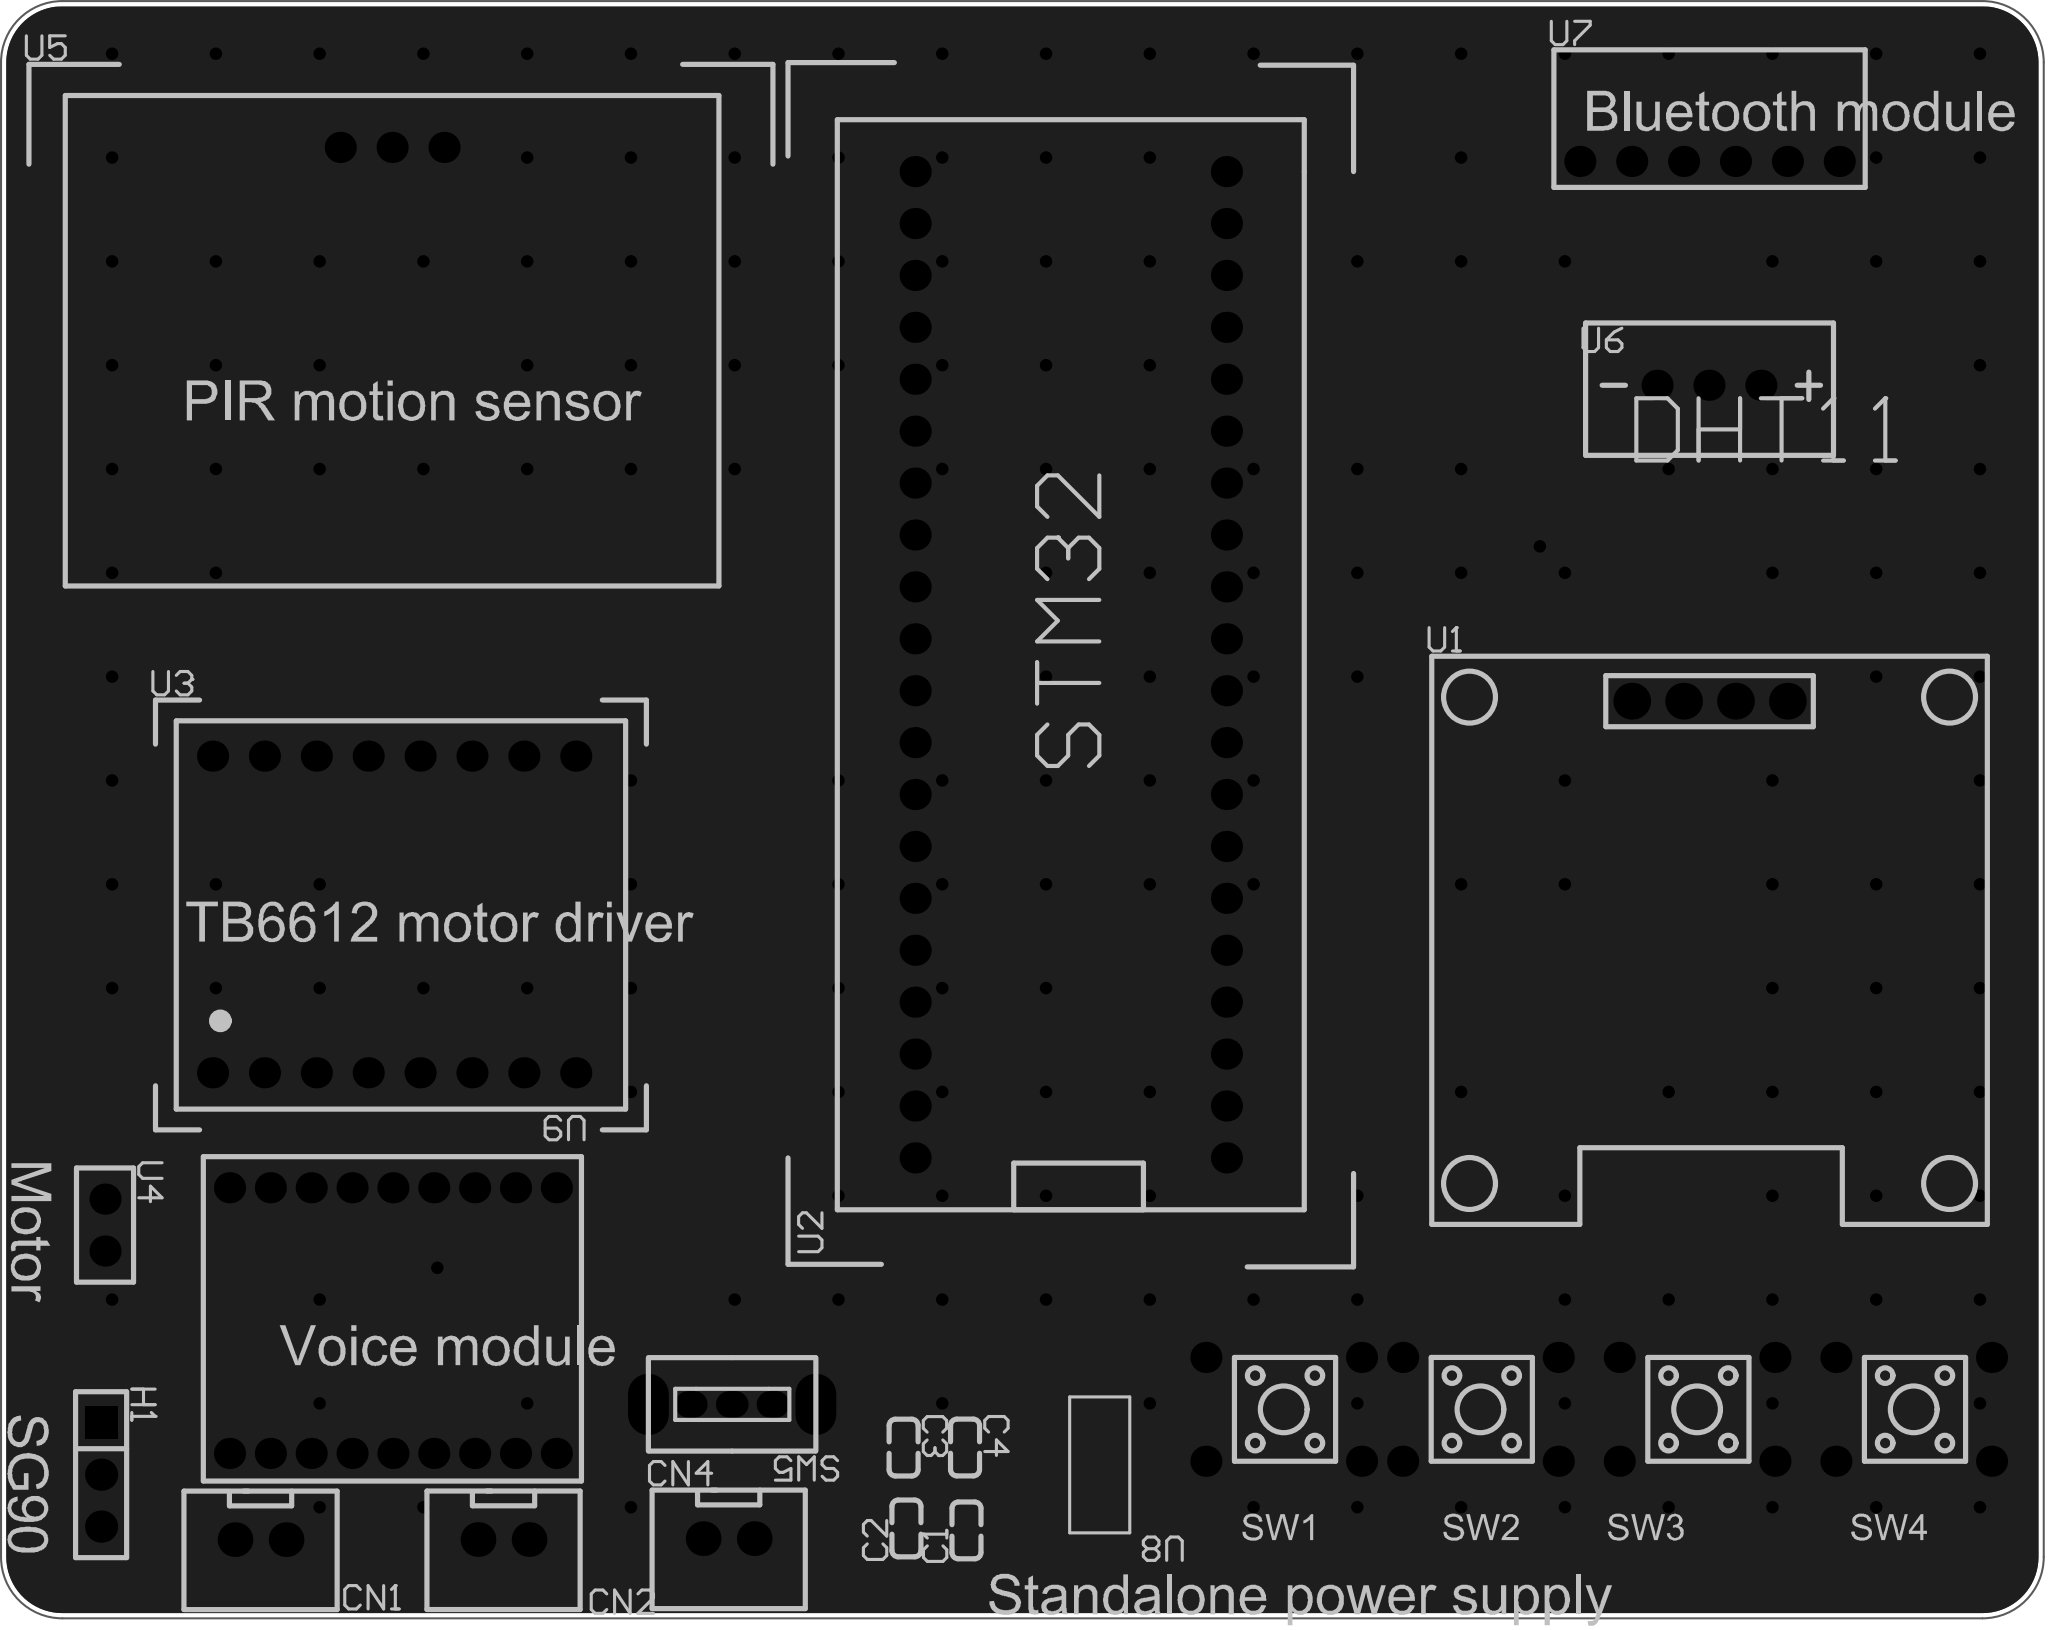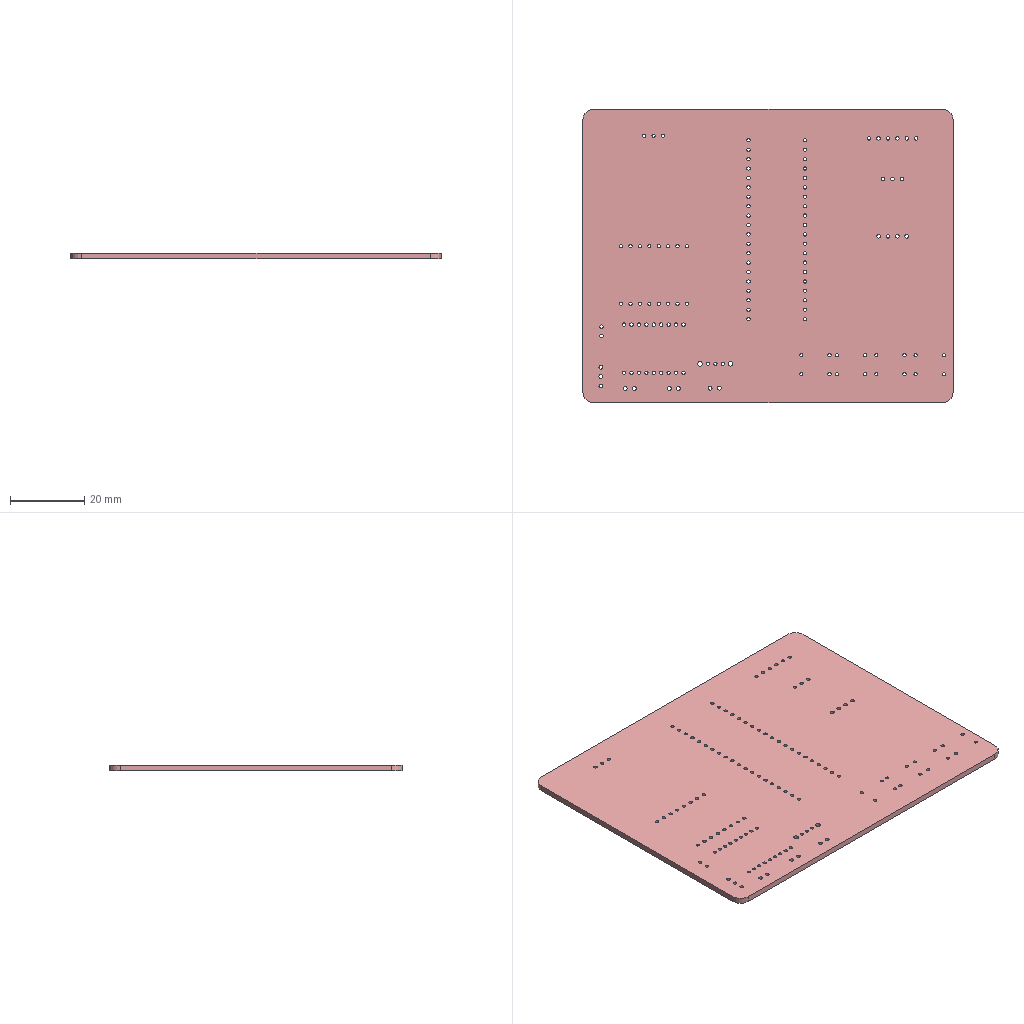Circuit board layout | Altium Designer | box 100 x 79.1 x 1.6 mm
Layer stack:
# Altium Designer layer stack of  (unit mm; dielectric type: 0 none, 1 core, 2 prepreg, 3 surface material)
index,name,kind,layer,copper_thickness_mm,dielectric_type,dielectric_thickness_mm,dielectric_material,dielectric_constant
0,Top Paste Mask Layer,other,,,,,,
1,Top Silkscreen Layer,other,,,,,,
2,Top Solder Mask Layer,dielectric,,,3,0.01,,3.3
3,Top Layer,copper,Top Layer,0.035,,,,
4,Dielectric1,dielectric,,,3,1.51,FR4,4.5
5,Bottom Layer,copper,Bottom Layer,0.035,,,,
6,Bottom Solder Mask Layer,dielectric,,,3,0.01,,3.3
7,Bottom Silkscreen Layer,other,,,,,,
8,Bottom Paste Mask Layer,other,,,,,,
# drill layer pairs: low layer,high layer
drill_pair,Top Layer,Bottom Layer
Part placement:
Designator,Comment,Layer,Footprint,Center-X(mm),Center-Y(mm),Rotation
U1,HS96L03W2C03,TopLayer,OLED-TH_L27.8-W27.2-P2.54_C9900033791,159.84,121.796,0
U2,,TopLayer,STM32,128.57,123.579,90
U3,,TopLayer,电机驱动模块,95.445,111.36,0
U4,,TopLayer,直流电机,81.291,96.162,270
U5,,TopLayer,人体红外模块,95.347,148.892,0
U6,,TopLayer,DHT11温湿度,159.812,137.254,0
SW1,,TopLayer,按键,138.994,87.145,90
SW2,,TopLayer,按键,148.626,87.145,90
SW3,,TopLayer,按键,159.23,87.145,90
U7,,TopLayer,蓝牙HC-08,159.84,148.207,0
SW4,,TopLayer,按键,169.835,87.145,90
C1,100nF,TopLayer,C0603,123.463,81.221,90
C2,10uF,TopLayer,C0603,120.524,81.317,90
C3,100nF,TopLayer,C0603,120.385,85.273,270
C4,10uF,TopLayer,C0603,123.393,85.277,270
CN1,XH2.54*2P_through-hole,TopLayer,CONN-TH_2P-P2.50-XH2.54-2P,88.904,80.77,0
CN2,XH2.54*2P_through-hole,TopLayer,CONN-TH_2P-P2.50-XH2.54-2P,100.8,80.773,0
CN4,XH2.54*2P_through-hole,TopLayer,CONN-TH_2P-P2.50-XH2.54-2P,111.822,80.819,0
H1,,TopLayer,HDR-TH_3P-P2.54-V-F,81.099,83.948,270
SW5,,TopLayer,拨动开关,111.99,87.388,180
U8,AMS1117-3.3,TopLayer,SOT-223-3_L6.5-W3.4-P2.30-LS7.0-BR,129.886,84.427,180
U9,CON2.0MM-PAD-18,TopLayer,CONN-TH_18P-P2.00_C9900078766,95.385,91.488,180
Pad and via stacks:
# Altium Designer via and pad stacks of  (unit mm). Each distinct definition once, with the count of objects using it.
# via: kind,start_layer,end_layer,hole_mm,diameter_mm,mode(0 simple;1 top-mid-bottom;2 full stack),diameter_per_layer,count,example_net
# pad: kind,layer,hole_mm,hole_type(0 round;1 square;2 slot),plating,top_size,top_shape(1 round;2 rect;3 octagon;9 rounded rect),mid_size,bottom_size,mode,footprint,size_per_layer,count,example
pad,Multi-Layer,1.05,0,plated,1.8x1.8,1,1.8x1.8,1.8x1.8,0,OLED-TH_L27.8-W27.2-P2.54_C9900033791,,4,U1.1
pad,Multi-Layer,0.9144,0,plated,1.524x1.524,1,1.524x1.524,1.524x1.524,0,STM32,,40,U2.1
pad,Multi-Layer,0.9144,0,plated,1.524x1.524,1,1.524x1.524,1.524x1.524,0,\u00B5\u00E7\u00BB\u00FA\u00C7\u00FD\u00B6\u00AF\u00C4\u00A3\u00BF\u00E9,,16,U3.1
pad,Multi-Layer,0.9144,0,plated,1.524x1.524,1,1.524x1.524,1.524x1.524,0,\u00D6\u00B1\u00C1\u00F7\u00B5\u00E7\u00BB\u00FA,,2,U4.1
pad,Multi-Layer,0.9144,0,plated,1.524x1.524,1,1.524x1.524,1.524x1.524,0,\u00C8\u00CB\u00CC\u00E5\u00BA\u00EC\u00CD\u00E2\u00C4\u00A3\u00BF\u00E9,,3,U5.1
pad,Multi-Layer,0.9144,0,plated,1.524x1.524,1,1.524x1.524,1.524x1.524,0,DHT11\u00CE\u00C2\u00CA\u00AA\u00B6\u00C8,,3,U6.3
pad,Multi-Layer,0.9144,0,plated,1.524x1.524,1,1.524x1.524,1.524x1.524,0,\u00B0\u00B4\u00BC\u00FC,,16,SW1.1
pad,Multi-Layer,0.9144,0,plated,1.524x1.524,1,1.524x1.524,1.524x1.524,0,\u00C0\u00B6\u00D1\u00C0HC-08,,6,U7.1
pad,Multi-Layer,1.05,0,plated,1.7x1.7,1,1.7x1.7,1.7x1.7,0,CONN-TH_2P-P2.50-XH2.54-2P,,6,CN1.2
pad,Multi-Layer,1.02,0,plated,1.575x1.575,1,1.575x1.575,1.575x1.575,0,HDR-TH_3P-P2.54-V-F,,2,H1.3
pad,Multi-Layer,1.02,0,plated,1.575x1.575,2,1.575x1.575,1.575x1.575,0,HDR-TH_3P-P2.54-V-F,,1,H1.1
pad,Multi-Layer,0.8992,0,plated,1.6x1.3,1,1.6x1.3,1.6x1.3,0,\u00B2\u00A6\u00B6\u00AF\u00BF\u00AA\u00B9\u00D8,,3,SW5.1
pad,Multi-Layer,1.3,0,plated,3x1.999,1,3x1.999,3x1.999,0,\u00B2\u00A6\u00B6\u00AF\u00BF\u00AA\u00B9\u00D8,,2,SW5.4
pad,Multi-Layer,0.9,0,plated,1.524x1.524,1,1.524x1.524,1.524x1.524,0,CONN-TH_18P-P2.00_C9900078766,,18,U9.1
pad,Top Layer,0,0,plated,0.8x0.9,2,0.8x0.9,0.8x0.9,0,C0603,,8,C1.2
pad,Top Layer,0,0,plated,2.5x1.1,2,2.5x1.1,2.5x1.1,0,SOT-223-3_L6.5-W3.4-P2.30-LS7.0-BR,,3,U8.1
pad,Top Layer,0,0,plated,2.34x3.6,2,2.34x3.6,2.34x3.6,0,SOT-223-3_L6.5-W3.4-P2.30-LS7.0-BR,,1,U8.4
via,Top Layer,Bottom Layer,0.3048,0.61,0,,183,PA10
Copper pours:
name,layer,net,type(0 solid;1 hatched;2 none)
Bottom Layer-GND,Bottom Layer,GND,0
Top Layer-GND,Top Layer,GND,0
Design rules, without the lines most boards share:
# Altium Designer design rules of  (exported by Altium Designer, unit mm)
# columns: name | kind | enabled | priority | scope1 | scope2 | descriptor | typed fields (field=value)
otherClearance | 52 | enabled | 1 | All | All | Hole To Hole Clearance (Gap=11.8mil) (All),(All) | gap=0.2997